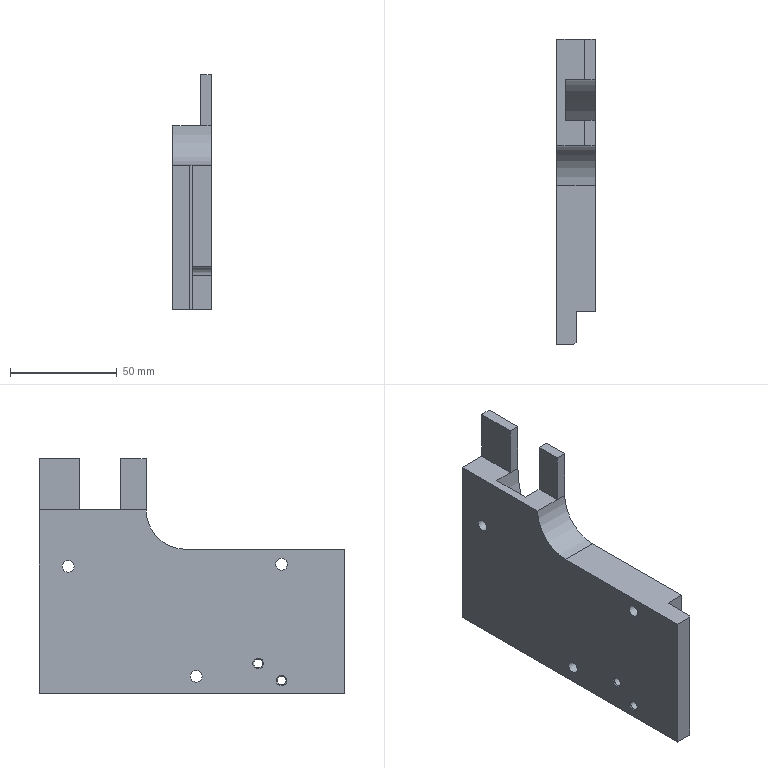Part | STEP file | 1 solid | 51 faces | box 18 x 143 x 110 mm | volume 148333 mm3 | plane 25 | cylinder 16 | cone 10 | commonest cylinder face diameters 4.134 x4 5.5 x3 10 x3 6.647 x1 8 x1 19 x1